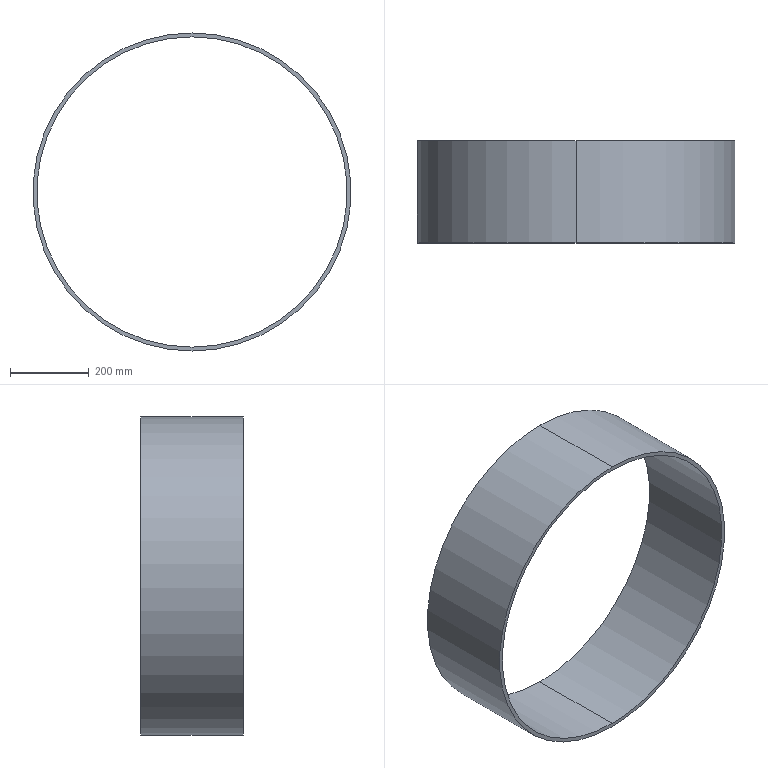Part | SolidWorks | features Extrusion 1 | 1 solid | 6 faces | box 810 x 260 x 810 mm | volume 6534513 mm3 | cylinder 4 | plane 2 | commonest cylinder face diameters 790 x2 810 x2
STEP:
#1=CARTESIAN_POINT('',(0.,260.,-395.));
#2=VERTEX_POINT('',#1);
#3=CARTESIAN_POINT('',(0.,260.,395.));
#4=VERTEX_POINT('',#3);
#5=CARTESIAN_POINT('',(0.,260.,0.));
#6=DIRECTION('',(0.,1.,0.));
#7=DIRECTION('',(0.,0.,1.));
#8=AXIS2_PLACEMENT_3D('',#5,#6,#7);
#9=CIRCLE('',#8,395.);
#10=EDGE_CURVE('',#2,#4,#9,.T.);
#11=ORIENTED_EDGE('',*,*,#10,.T.);
#12=CARTESIAN_POINT('',(0.,0.,395.));
#13=VERTEX_POINT('',#12);
#14=CARTESIAN_POINT('',(0.,260.,395.));
#15=DIRECTION('',(0.,-1.,0.));
#16=VECTOR('',#15,1000.);
#17=LINE('',#14,#16);
#18=EDGE_CURVE('',#4,#13,#17,.T.);
#19=ORIENTED_EDGE('',*,*,#18,.T.);
#20=CARTESIAN_POINT('',(0.,0.,-395.));
#21=VERTEX_POINT('',#20);
#22=CARTESIAN_POINT('',(0.,0.,0.));
#23=DIRECTION('',(0.,1.,0.));
#24=DIRECTION('',(0.,0.,1.));
#25=AXIS2_PLACEMENT_3D('',#22,#23,#24);
#26=CIRCLE('',#25,395.);
#27=EDGE_CURVE('',#21,#13,#26,.T.);
#28=ORIENTED_EDGE('',*,*,#27,.F.);
#29=CARTESIAN_POINT('',(0.,260.,-395.));
#30=DIRECTION('',(0.,-1.,0.));
#31=VECTOR('',#30,1000.);
#32=LINE('',#29,#31);
#33=EDGE_CURVE('',#2,#21,#32,.T.);
#34=ORIENTED_EDGE('',*,*,#33,.F.);
#35=EDGE_LOOP('',(#11,#19,#28,#34));
#36=FACE_OUTER_BOUND('',#35,.T.);
#37=CARTESIAN_POINT('',(0.,260.,0.));
#38=DIRECTION('',(0.,-1.,0.));
#39=DIRECTION('',(0.,0.,-1.));
#40=AXIS2_PLACEMENT_3D('',#37,#38,#39);
#41=CYLINDRICAL_SURFACE('',#40,395.);
#42=ADVANCED_FACE('',(#36),#41,.F.);
#43=CARTESIAN_POINT('',(0.,260.,405.));
#44=VERTEX_POINT('',#43);
#45=CARTESIAN_POINT('',(0.,260.,-405.));
#46=VERTEX_POINT('',#45);
#47=CARTESIAN_POINT('',(0.,260.,0.));
#48=DIRECTION('',(0.,1.,0.));
#49=DIRECTION('',(0.,0.,1.));
#50=AXIS2_PLACEMENT_3D('',#47,#48,#49);
#51=CIRCLE('',#50,405.);
#52=EDGE_CURVE('',#44,#46,#51,.T.);
#53=ORIENTED_EDGE('',*,*,#52,.F.);
#54=CARTESIAN_POINT('',(0.,0.,405.));
#55=VERTEX_POINT('',#54);
#56=CARTESIAN_POINT('',(0.,260.,405.));
#57=DIRECTION('',(0.,-1.,0.));
#58=VECTOR('',#57,1000.);
#59=LINE('',#56,#58);
#60=EDGE_CURVE('',#44,#55,#59,.T.);
#61=ORIENTED_EDGE('',*,*,#60,.T.);
#62=CARTESIAN_POINT('',(0.,0.,-405.));
#63=VERTEX_POINT('',#62);
#64=CARTESIAN_POINT('',(0.,0.,0.));
#65=DIRECTION('',(0.,1.,0.));
#66=DIRECTION('',(0.,0.,1.));
#67=AXIS2_PLACEMENT_3D('',#64,#65,#66);
#68=CIRCLE('',#67,405.);
#69=EDGE_CURVE('',#55,#63,#68,.T.);
#70=ORIENTED_EDGE('',*,*,#69,.T.);
#71=CARTESIAN_POINT('',(0.,260.,-405.));
#72=DIRECTION('',(0.,-1.,0.));
#73=VECTOR('',#72,1000.);
#74=LINE('',#71,#73);
#75=EDGE_CURVE('',#46,#63,#74,.T.);
#76=ORIENTED_EDGE('',*,*,#75,.F.);
#77=EDGE_LOOP('',(#53,#61,#70,#76));
#78=FACE_OUTER_BOUND('',#77,.T.);
#79=CARTESIAN_POINT('',(0.,260.,0.));
#80=DIRECTION('',(0.,-1.,0.));
#81=DIRECTION('',(0.,0.,-1.));
#82=AXIS2_PLACEMENT_3D('',#79,#80,#81);
#83=CYLINDRICAL_SURFACE('',#82,405.);
#84=ADVANCED_FACE('',(#78),#83,.T.);
#85=CARTESIAN_POINT('',(0.,260.,0.));
#86=DIRECTION('',(0.,1.,0.));
#87=DIRECTION('',(0.,0.,1.));
#88=AXIS2_PLACEMENT_3D('',#85,#86,#87);
#89=CIRCLE('',#88,405.);
#90=EDGE_CURVE('',#46,#44,#89,.T.);
#91=ORIENTED_EDGE('',*,*,#90,.T.);
#92=ORIENTED_EDGE('',*,*,#52,.T.);
#93=EDGE_LOOP('',(#91,#92));
#94=FACE_OUTER_BOUND('',#93,.T.);
#95=ORIENTED_EDGE('',*,*,#10,.F.);
#96=CARTESIAN_POINT('',(0.,260.,0.));
#97=DIRECTION('',(0.,1.,0.));
#98=DIRECTION('',(0.,0.,1.));
#99=AXIS2_PLACEMENT_3D('',#96,#97,#98);
#100=CIRCLE('',#99,395.);
#101=EDGE_CURVE('',#4,#2,#100,.T.);
#102=ORIENTED_EDGE('',*,*,#101,.F.);
#103=EDGE_LOOP('',(#95,#102));
#104=FACE_BOUND('',#103,.T.);
#105=CARTESIAN_POINT('',(0.,260.,0.));
#106=DIRECTION('',(0.,1.,0.));
#107=DIRECTION('',(0.,0.,1.));
#108=AXIS2_PLACEMENT_3D('',#105,#106,#107);
#109=PLANE('',#108);
#110=ADVANCED_FACE('',(#94,#104),#109,.T.);
#111=CARTESIAN_POINT('',(0.,0.,0.));
#112=DIRECTION('',(0.,1.,0.));
#113=DIRECTION('',(0.,0.,1.));
#114=AXIS2_PLACEMENT_3D('',#111,#112,#113);
#115=CIRCLE('',#114,405.);
#116=EDGE_CURVE('',#63,#55,#115,.T.);
#117=ORIENTED_EDGE('',*,*,#116,.F.);
#118=ORIENTED_EDGE('',*,*,#69,.F.);
#119=EDGE_LOOP('',(#117,#118));
#120=FACE_OUTER_BOUND('',#119,.T.);
#121=ORIENTED_EDGE('',*,*,#27,.T.);
#122=CARTESIAN_POINT('',(0.,0.,0.));
#123=DIRECTION('',(0.,1.,0.));
#124=DIRECTION('',(0.,0.,1.));
#125=AXIS2_PLACEMENT_3D('',#122,#123,#124);
#126=CIRCLE('',#125,395.);
#127=EDGE_CURVE('',#13,#21,#126,.T.);
#128=ORIENTED_EDGE('',*,*,#127,.T.);
#129=EDGE_LOOP('',(#121,#128));
#130=FACE_BOUND('',#129,.T.);
#131=CARTESIAN_POINT('',(0.,0.,0.));
#132=DIRECTION('',(0.,1.,0.));
#133=DIRECTION('',(0.,0.,1.));
#134=AXIS2_PLACEMENT_3D('',#131,#132,#133);
#135=PLANE('',#134);
#136=ADVANCED_FACE('',(#120,#130),#135,.F.);
#137=ORIENTED_EDGE('',*,*,#60,.F.);
#138=ORIENTED_EDGE('',*,*,#90,.F.);
#139=ORIENTED_EDGE('',*,*,#75,.T.);
#140=ORIENTED_EDGE('',*,*,#116,.T.);
#141=EDGE_LOOP('',(#137,#138,#139,#140));
#142=FACE_OUTER_BOUND('',#141,.T.);
#143=CARTESIAN_POINT('',(0.,260.,0.));
#144=DIRECTION('',(0.,-1.,0.));
#145=DIRECTION('',(0.,0.,-1.));
#146=AXIS2_PLACEMENT_3D('',#143,#144,#145);
#147=CYLINDRICAL_SURFACE('',#146,405.);
#148=ADVANCED_FACE('',(#142),#147,.T.);
#149=ORIENTED_EDGE('',*,*,#18,.F.);
#150=ORIENTED_EDGE('',*,*,#101,.T.);
#151=ORIENTED_EDGE('',*,*,#33,.T.);
#152=ORIENTED_EDGE('',*,*,#127,.F.);
#153=EDGE_LOOP('',(#149,#150,#151,#152));
#154=FACE_OUTER_BOUND('',#153,.T.);
#155=CARTESIAN_POINT('',(0.,260.,0.));
#156=DIRECTION('',(0.,-1.,0.));
#157=DIRECTION('',(0.,0.,-1.));
#158=AXIS2_PLACEMENT_3D('',#155,#156,#157);
#159=CYLINDRICAL_SURFACE('',#158,395.);
#160=ADVANCED_FACE('',(#154),#159,.F.);
#161=CLOSED_SHELL('',(#42,#84,#110,#136,#148,#160));
#162=MANIFOLD_SOLID_BREP('',#161);
#163=CARTESIAN_POINT('',(0.,0.,0.));
#164=DIRECTION('',(0.,0.,1.));
#165=DIRECTION('',(1.,0.,0.));
#166=AXIS2_PLACEMENT_3D('',#163,#164,#165);
#167=(LENGTH_UNIT()NAMED_UNIT(*)SI_UNIT(.MILLI.,.METRE.));
#168=UNCERTAINTY_MEASURE_WITH_UNIT(LENGTH_MEASURE(0.00001),#167,'','');
#169=(NAMED_UNIT(*)PLANE_ANGLE_UNIT()SI_UNIT($,.RADIAN.));
#170=(NAMED_UNIT(*)SI_UNIT($,.STERADIAN.)SOLID_ANGLE_UNIT());
#171=(GEOMETRIC_REPRESENTATION_CONTEXT(3)GLOBAL_UNCERTAINTY_ASSIGNED_CONTEXT((#168))GLOBAL_UNIT_ASSIGNED_CONTEXT((#167,#169,#170))REPRESENTATION_CONTEXT('',''));
#172=ADVANCED_BREP_SHAPE_REPRESENTATION('',(#162,#166),#171);